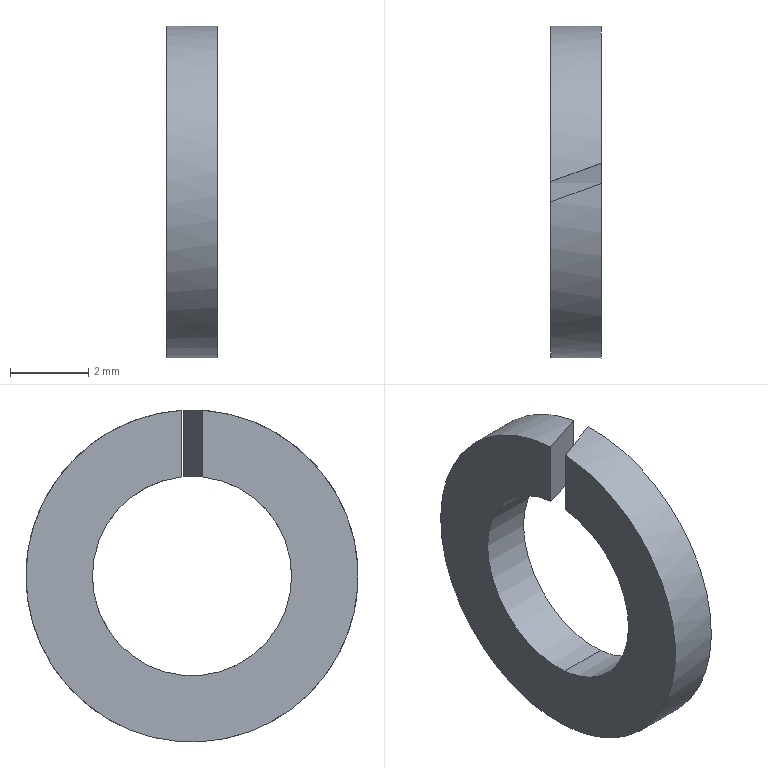Part | STEP file | KS B 1324 - No. 2 - 5 | 1 solid | 8 faces | box 1.3 x 8.5 x 8.5 mm | volume 46.057 mm3 | cylinder 4 | plane 4 | commonest cylinder face diameters 5.1 x2 8.5 x2
STEP:
#1=CARTESIAN_POINT('',(0.,0.,0.));
#2=DIRECTION('',(0.,0.,1.));
#3=DIRECTION('',(1.,0.,0.));
#4=AXIS2_PLACEMENT_3D('',#1,#2,#3);
#5=CARTESIAN_POINT('',(1.3,0.7332,2.442));
#6=VERTEX_POINT('',#5);
#7=CARTESIAN_POINT('',(0.,0.26,2.537));
#8=VERTEX_POINT('',#7);
#9=CARTESIAN_POINT('',(1.3,0.7332,2.442));
#10=CARTESIAN_POINT('',(0.8755,0.5787,2.489));
#11=CARTESIAN_POINT('',(0.4409,0.4205,2.52));
#12=CARTESIAN_POINT('',(0.,0.26,2.537));
#13=(BOUNDED_CURVE()B_SPLINE_CURVE(3,(#9,#10,#11,#12),.UNSPECIFIED.,.F.,.F.)B_SPLINE_CURVE_WITH_KNOTS((4,4),(4.421,4.61),.PIECEWISE_BEZIER_KNOTS.)CURVE()GEOMETRIC_REPRESENTATION_ITEM()RATIONAL_B_SPLINE_CURVE((1.,0.997,0.997,1.))REPRESENTATION_ITEM(''));
#14=CARTESIAN_POINT('',(0.,0.,0.));
#15=DIRECTION('',(1.,0.,0.));
#16=DIRECTION('',(0.,-0.09278,-0.9957));
#17=AXIS2_PLACEMENT_3D('',#14,#15,#16);
#18=CYLINDRICAL_SURFACE('',#17,2.55);
#19=CARTESIAN_POINT('',(2.943,1.3));
#20=CARTESIAN_POINT('',(2.946,1.281));
#21=CARTESIAN_POINT('',(2.951,1.242));
#22=CARTESIAN_POINT('',(2.96,1.184));
#23=CARTESIAN_POINT('',(2.969,1.126));
#24=CARTESIAN_POINT('',(2.977,1.068));
#25=CARTESIAN_POINT('',(2.986,1.009));
#26=CARTESIAN_POINT('',(2.995,0.9509));
#27=CARTESIAN_POINT('',(3.003,0.8922));
#28=CARTESIAN_POINT('',(3.012,0.8334));
#29=CARTESIAN_POINT('',(3.02,0.7744));
#30=CARTESIAN_POINT('',(3.029,0.7153));
#31=CARTESIAN_POINT('',(3.038,0.6562));
#32=CARTESIAN_POINT('',(3.046,0.5969));
#33=CARTESIAN_POINT('',(3.055,0.5375));
#34=CARTESIAN_POINT('',(3.063,0.4781));
#35=CARTESIAN_POINT('',(3.072,0.4185));
#36=CARTESIAN_POINT('',(3.081,0.3589));
#37=CARTESIAN_POINT('',(3.089,0.2992));
#38=CARTESIAN_POINT('',(3.098,0.2395));
#39=CARTESIAN_POINT('',(3.107,0.1797));
#40=CARTESIAN_POINT('',(3.115,0.1198));
#41=CARTESIAN_POINT('',(3.124,0.05993));
#42=CARTESIAN_POINT('',(3.13,0.01998));
#43=CARTESIAN_POINT('',(3.132,0.));
#44=B_SPLINE_CURVE_WITH_KNOTS('',3,(#19,#20,#21,#22,#23,#24,#25,#26,#27,#28,#29,#30,#31,#32,#33,#34,#35,#36,#37,#38,#39,#40,#41,#42,#43),.UNSPECIFIED.,.F.,.F.,(4,1,1,1,1,1,1,1,1,1,1,1,1,1,1,1,1,1,1,1,1,1,4),(4.421,4.429,4.438,4.447,4.455,4.464,4.472,4.481,4.49,4.498,4.507,4.516,4.524,4.533,4.541,4.55,4.559,4.567,4.576,4.584,4.593,4.602,4.61),.QUASI_UNIFORM_KNOTS.);
#45=(GEOMETRIC_REPRESENTATION_CONTEXT(2)PARAMETRIC_REPRESENTATION_CONTEXT()REPRESENTATION_CONTEXT('',''));
#46=DEFINITIONAL_REPRESENTATION('',(#44),#45);
#47=PCURVE('',#18,#46);
#48=CARTESIAN_POINT('',(0.,0.26,0.));
#49=DIRECTION('',(-0.342,0.9397,0.));
#50=DIRECTION('',(0.,0.,1.));
#51=AXIS2_PLACEMENT_3D('',#48,#49,#50);
#52=PLANE('',#51);
#53=CARTESIAN_POINT('',(2.442,1.383));
#54=CARTESIAN_POINT('',(2.489,0.9317));
#55=CARTESIAN_POINT('',(2.52,0.4692));
#56=CARTESIAN_POINT('',(2.537,0.));
#57=(BOUNDED_CURVE()B_SPLINE_CURVE(3,(#53,#54,#55,#56),.UNSPECIFIED.,.F.,.F.)B_SPLINE_CURVE_WITH_KNOTS((4,4),(4.421,4.61),.PIECEWISE_BEZIER_KNOTS.)CURVE()GEOMETRIC_REPRESENTATION_ITEM()RATIONAL_B_SPLINE_CURVE((1.,0.997,0.997,1.))REPRESENTATION_ITEM(''));
#58=(GEOMETRIC_REPRESENTATION_CONTEXT(2)PARAMETRIC_REPRESENTATION_CONTEXT()REPRESENTATION_CONTEXT('',''));
#59=DEFINITIONAL_REPRESENTATION('',(#57),#58);
#60=PCURVE('',#52,#59);
#61=SURFACE_CURVE('',#13,(#47,#60),.PCURVE_S1.);
#62=EDGE_CURVE('',#6,#8,#61,.T.);
#63=ORIENTED_EDGE('',*,*,#62,.F.);
#64=CARTESIAN_POINT('',(1.3,-0.2366,-2.539));
#65=VERTEX_POINT('',#64);
#66=CARTESIAN_POINT('',(1.3,0.,0.));
#67=DIRECTION('',(-1.,0.,0.));
#68=DIRECTION('',(0.,-1.,0.));
#69=AXIS2_PLACEMENT_3D('',#66,#67,#68);
#70=CIRCLE('',#69,2.55);
#71=CARTESIAN_POINT('',(4.805,1.3));
#72=DIRECTION('',(-1.,0.));
#73=VECTOR('',#72,1.);
#74=LINE('',#71,#73);
#75=(GEOMETRIC_REPRESENTATION_CONTEXT(2)PARAMETRIC_REPRESENTATION_CONTEXT()REPRESENTATION_CONTEXT('',''));
#76=DEFINITIONAL_REPRESENTATION('',(#74),#75);
#77=PCURVE('',#18,#76);
#78=CARTESIAN_POINT('',(1.3,0.,0.));
#79=DIRECTION('',(-1.,0.,0.));
#80=DIRECTION('',(0.,0.,1.));
#81=AXIS2_PLACEMENT_3D('',#78,#79,#80);
#82=PLANE('',#81);
#83=CARTESIAN_POINT('',(0.,0.));
#84=DIRECTION('',(0.,-1.));
#85=AXIS2_PLACEMENT_2D('',#83,#84);
#86=CIRCLE('',#85,2.55);
#87=(GEOMETRIC_REPRESENTATION_CONTEXT(2)PARAMETRIC_REPRESENTATION_CONTEXT()REPRESENTATION_CONTEXT('',''));
#88=DEFINITIONAL_REPRESENTATION('',(#86),#87);
#89=PCURVE('',#82,#88);
#90=SURFACE_CURVE('',#70,(#77,#89),.PCURVE_S1.);
#91=EDGE_CURVE('',#6,#65,#90,.T.);
#92=ORIENTED_EDGE('',*,*,#91,.T.);
#93=CARTESIAN_POINT('',(0.,-0.2366,-2.539));
#94=VERTEX_POINT('',#93);
#95=CARTESIAN_POINT('',(0.,-0.2366,-2.539));
#96=DIRECTION('',(1.,0.,0.));
#97=VECTOR('',#96,1.);
#98=LINE('',#95,#97);
#99=CARTESIAN_POINT('',(0.,0.));
#100=DIRECTION('',(0.,1.));
#101=VECTOR('',#100,1.);
#102=LINE('',#99,#101);
#103=(GEOMETRIC_REPRESENTATION_CONTEXT(2)PARAMETRIC_REPRESENTATION_CONTEXT()REPRESENTATION_CONTEXT('',''));
#104=DEFINITIONAL_REPRESENTATION('',(#102),#103);
#105=PCURVE('',#18,#104);
#106=CARTESIAN_POINT('',(0.,0.,0.));
#107=DIRECTION('',(1.,0.,0.));
#108=DIRECTION('',(0.,-0.09278,-0.9957));
#109=AXIS2_PLACEMENT_3D('',#106,#107,#108);
#110=CYLINDRICAL_SURFACE('',#109,2.55);
#111=CARTESIAN_POINT('',(6.283,0.));
#112=DIRECTION('',(0.,1.));
#113=VECTOR('',#112,1.);
#114=LINE('',#111,#113);
#115=(GEOMETRIC_REPRESENTATION_CONTEXT(2)PARAMETRIC_REPRESENTATION_CONTEXT()REPRESENTATION_CONTEXT('',''));
#116=DEFINITIONAL_REPRESENTATION('',(#114),#115);
#117=PCURVE('',#110,#116);
#118=SURFACE_CURVE('',#98,(#105,#117),.PCURVE_S1.);
#119=EDGE_CURVE('',#94,#65,#118,.T.);
#120=ORIENTED_EDGE('',*,*,#119,.F.);
#121=CARTESIAN_POINT('',(0.,0.,0.));
#122=DIRECTION('',(1.,0.,0.));
#123=DIRECTION('',(0.,-1.,0.));
#124=AXIS2_PLACEMENT_3D('',#121,#122,#123);
#125=CIRCLE('',#124,2.55);
#126=CARTESIAN_POINT('',(-1.478,0.));
#127=DIRECTION('',(1.,0.));
#128=VECTOR('',#127,1.);
#129=LINE('',#126,#128);
#130=(GEOMETRIC_REPRESENTATION_CONTEXT(2)PARAMETRIC_REPRESENTATION_CONTEXT()REPRESENTATION_CONTEXT('',''));
#131=DEFINITIONAL_REPRESENTATION('',(#129),#130);
#132=PCURVE('',#18,#131);
#133=CARTESIAN_POINT('',(0.,0.,0.));
#134=DIRECTION('',(-1.,0.,0.));
#135=DIRECTION('',(0.,0.,1.));
#136=AXIS2_PLACEMENT_3D('',#133,#134,#135);
#137=PLANE('',#136);
#138=CARTESIAN_POINT('',(0.,-2.55));
#139=CARTESIAN_POINT('',(-4.417,-2.55));
#140=CARTESIAN_POINT('',(-2.208,1.275));
#141=CARTESIAN_POINT('',(0.,5.1));
#142=CARTESIAN_POINT('',(2.208,1.275));
#143=CARTESIAN_POINT('',(4.417,-2.55));
#144=CARTESIAN_POINT('',(0.,-2.55));
#145=(BOUNDED_CURVE()B_SPLINE_CURVE(2,(#138,#139,#140,#141,#142,#143,#144),.UNSPECIFIED.,.T.,.F.)B_SPLINE_CURVE_WITH_KNOTS((1,2,2,2,2,1),(-2.094,0.,2.094,4.189,6.283,8.378),.UNSPECIFIED.)CURVE()GEOMETRIC_REPRESENTATION_ITEM()RATIONAL_B_SPLINE_CURVE((1.,0.5,1.,0.5,1.,0.5,1.))REPRESENTATION_ITEM(''));
#146=(GEOMETRIC_REPRESENTATION_CONTEXT(2)PARAMETRIC_REPRESENTATION_CONTEXT()REPRESENTATION_CONTEXT('',''));
#147=DEFINITIONAL_REPRESENTATION('',(#145),#146);
#148=PCURVE('',#137,#147);
#149=SURFACE_CURVE('',#125,(#132,#148),.PCURVE_S1.);
#150=EDGE_CURVE('',#94,#8,#149,.T.);
#151=ORIENTED_EDGE('',*,*,#150,.T.);
#152=EDGE_LOOP('',(#63,#92,#120,#151));
#153=FACE_BOUND('',#152,.F.);
#154=ADVANCED_FACE('',(#153),#18,.F.);
#155=CARTESIAN_POINT('',(0.,-0.2366,-4.243));
#156=VERTEX_POINT('',#155);
#157=CARTESIAN_POINT('',(0.,-0.26,4.242));
#158=VERTEX_POINT('',#157);
#159=CARTESIAN_POINT('',(0.,0.,0.));
#160=DIRECTION('',(-1.,0.,0.));
#161=DIRECTION('',(0.,-1.,0.));
#162=AXIS2_PLACEMENT_3D('',#159,#160,#161);
#163=CIRCLE('',#162,4.25);
#164=CARTESIAN_POINT('',(0.,0.,0.));
#165=DIRECTION('',(1.,0.,0.));
#166=DIRECTION('',(0.,-0.05567,-0.9984));
#167=AXIS2_PLACEMENT_3D('',#164,#165,#166);
#168=CYLINDRICAL_SURFACE('',#167,4.25);
#169=CARTESIAN_POINT('',(11.051,0.));
#170=DIRECTION('',(-1.,0.));
#171=VECTOR('',#170,1.);
#172=LINE('',#169,#171);
#173=(GEOMETRIC_REPRESENTATION_CONTEXT(2)PARAMETRIC_REPRESENTATION_CONTEXT()REPRESENTATION_CONTEXT('',''));
#174=DEFINITIONAL_REPRESENTATION('',(#172),#173);
#175=PCURVE('',#168,#174);
#176=CARTESIAN_POINT('',(0.,0.));
#177=DIRECTION('',(0.,-1.));
#178=AXIS2_PLACEMENT_2D('',#176,#177);
#179=CIRCLE('',#178,4.25);
#180=(GEOMETRIC_REPRESENTATION_CONTEXT(2)PARAMETRIC_REPRESENTATION_CONTEXT()REPRESENTATION_CONTEXT('',''));
#181=DEFINITIONAL_REPRESENTATION('',(#179),#180);
#182=PCURVE('',#137,#181);
#183=SURFACE_CURVE('',#163,(#175,#182),.PCURVE_S1.);
#184=EDGE_CURVE('',#156,#158,#183,.T.);
#185=ORIENTED_EDGE('',*,*,#184,.F.);
#186=CARTESIAN_POINT('',(1.3,-0.2366,-4.243));
#187=VERTEX_POINT('',#186);
#188=CARTESIAN_POINT('',(0.,-0.2366,-4.243));
#189=DIRECTION('',(1.,0.,0.));
#190=VECTOR('',#189,1.);
#191=LINE('',#188,#190);
#192=CARTESIAN_POINT('',(6.283,0.));
#193=DIRECTION('',(0.,1.));
#194=VECTOR('',#193,1.);
#195=LINE('',#192,#194);
#196=(GEOMETRIC_REPRESENTATION_CONTEXT(2)PARAMETRIC_REPRESENTATION_CONTEXT()REPRESENTATION_CONTEXT('',''));
#197=DEFINITIONAL_REPRESENTATION('',(#195),#196);
#198=PCURVE('',#168,#197);
#199=CARTESIAN_POINT('',(0.,0.,0.));
#200=DIRECTION('',(1.,0.,0.));
#201=DIRECTION('',(0.,-0.05567,-0.9984));
#202=AXIS2_PLACEMENT_3D('',#199,#200,#201);
#203=CYLINDRICAL_SURFACE('',#202,4.25);
#204=CARTESIAN_POINT('',(0.,0.));
#205=DIRECTION('',(0.,1.));
#206=VECTOR('',#205,1.);
#207=LINE('',#204,#206);
#208=(GEOMETRIC_REPRESENTATION_CONTEXT(2)PARAMETRIC_REPRESENTATION_CONTEXT()REPRESENTATION_CONTEXT('',''));
#209=DEFINITIONAL_REPRESENTATION('',(#207),#208);
#210=PCURVE('',#203,#209);
#211=SURFACE_CURVE('',#191,(#198,#210),.PCURVE_S1.);
#212=EDGE_CURVE('',#156,#187,#211,.T.);
#213=ORIENTED_EDGE('',*,*,#212,.T.);
#214=CARTESIAN_POINT('',(1.3,0.2132,4.245));
#215=VERTEX_POINT('',#214);
#216=CARTESIAN_POINT('',(1.3,0.,0.));
#217=DIRECTION('',(-1.,0.,0.));
#218=DIRECTION('',(0.,-1.,0.));
#219=AXIS2_PLACEMENT_3D('',#216,#217,#218);
#220=CIRCLE('',#219,4.25);
#221=CARTESIAN_POINT('',(11.051,1.3));
#222=DIRECTION('',(-1.,0.));
#223=VECTOR('',#222,1.);
#224=LINE('',#221,#223);
#225=(GEOMETRIC_REPRESENTATION_CONTEXT(2)PARAMETRIC_REPRESENTATION_CONTEXT()REPRESENTATION_CONTEXT('',''));
#226=DEFINITIONAL_REPRESENTATION('',(#224),#225);
#227=PCURVE('',#168,#226);
#228=CARTESIAN_POINT('',(0.,0.));
#229=DIRECTION('',(0.,-1.));
#230=AXIS2_PLACEMENT_2D('',#228,#229);
#231=CIRCLE('',#230,4.25);
#232=(GEOMETRIC_REPRESENTATION_CONTEXT(2)PARAMETRIC_REPRESENTATION_CONTEXT()REPRESENTATION_CONTEXT('',''));
#233=DEFINITIONAL_REPRESENTATION('',(#231),#232);
#234=PCURVE('',#82,#233);
#235=SURFACE_CURVE('',#220,(#227,#234),.PCURVE_S1.);
#236=EDGE_CURVE('',#187,#215,#235,.T.);
#237=ORIENTED_EDGE('',*,*,#236,.T.);
#238=CARTESIAN_POINT('',(1.3,0.2132,4.245));
#239=CARTESIAN_POINT('',(0.8668,0.05547,4.253));
#240=CARTESIAN_POINT('',(0.433,-0.1024,4.252));
#241=CARTESIAN_POINT('',(0.,-0.26,4.242));
#242=(BOUNDED_CURVE()B_SPLINE_CURVE(3,(#238,#239,#240,#241),.UNSPECIFIED.,.F.,.F.)B_SPLINE_CURVE_WITH_KNOTS((4,4),(4.662,4.774),.PIECEWISE_BEZIER_KNOTS.)CURVE()GEOMETRIC_REPRESENTATION_ITEM()RATIONAL_B_SPLINE_CURVE((1.,0.999,0.999,1.))REPRESENTATION_ITEM(''));
#243=CARTESIAN_POINT('',(3.147,1.3));
#244=CARTESIAN_POINT('',(3.149,1.28));
#245=CARTESIAN_POINT('',(3.152,1.241));
#246=CARTESIAN_POINT('',(3.157,1.182));
#247=CARTESIAN_POINT('',(3.162,1.123));
#248=CARTESIAN_POINT('',(3.167,1.064));
#249=CARTESIAN_POINT('',(3.172,1.005));
#250=CARTESIAN_POINT('',(3.177,0.9456));
#251=CARTESIAN_POINT('',(3.183,0.8864));
#252=CARTESIAN_POINT('',(3.188,0.8273));
#253=CARTESIAN_POINT('',(3.193,0.7682));
#254=CARTESIAN_POINT('',(3.198,0.709));
#255=CARTESIAN_POINT('',(3.203,0.6499));
#256=CARTESIAN_POINT('',(3.208,0.5908));
#257=CARTESIAN_POINT('',(3.213,0.5316));
#258=CARTESIAN_POINT('',(3.218,0.4725));
#259=CARTESIAN_POINT('',(3.223,0.4134));
#260=CARTESIAN_POINT('',(3.228,0.3543));
#261=CARTESIAN_POINT('',(3.233,0.2952));
#262=CARTESIAN_POINT('',(3.238,0.2361));
#263=CARTESIAN_POINT('',(3.243,0.177));
#264=CARTESIAN_POINT('',(3.248,0.118));
#265=CARTESIAN_POINT('',(3.253,0.05899));
#266=CARTESIAN_POINT('',(3.257,0.01966));
#267=CARTESIAN_POINT('',(3.259,0.));
#268=B_SPLINE_CURVE_WITH_KNOTS('',3,(#243,#244,#245,#246,#247,#248,#249,#250,#251,#252,#253,#254,#255,#256,#257,#258,#259,#260,#261,#262,#263,#264,#265,#266,#267),.UNSPECIFIED.,.F.,.F.,(4,1,1,1,1,1,1,1,1,1,1,1,1,1,1,1,1,1,1,1,1,1,4),(4.662,4.667,4.672,4.677,4.682,4.688,4.693,4.698,4.703,4.708,4.713,4.718,4.723,4.728,4.733,4.738,4.743,4.748,4.753,4.758,4.763,4.769,4.774),.QUASI_UNIFORM_KNOTS.);
#269=(GEOMETRIC_REPRESENTATION_CONTEXT(2)PARAMETRIC_REPRESENTATION_CONTEXT()REPRESENTATION_CONTEXT('',''));
#270=DEFINITIONAL_REPRESENTATION('',(#268),#269);
#271=PCURVE('',#168,#270);
#272=CARTESIAN_POINT('',(1.3,0.2132,0.));
#273=DIRECTION('',(0.342,-0.9397,0.));
#274=DIRECTION('',(0.,0.,-1.));
#275=AXIS2_PLACEMENT_3D('',#272,#273,#274);
#276=PLANE('',#275);
#277=CARTESIAN_POINT('',(-4.245,0.));
#278=CARTESIAN_POINT('',(-4.253,-0.461));
#279=CARTESIAN_POINT('',(-4.252,-0.9227));
#280=CARTESIAN_POINT('',(-4.242,-1.383));
#281=(BOUNDED_CURVE()B_SPLINE_CURVE(3,(#277,#278,#279,#280),.UNSPECIFIED.,.F.,.F.)B_SPLINE_CURVE_WITH_KNOTS((4,4),(4.662,4.774),.PIECEWISE_BEZIER_KNOTS.)CURVE()GEOMETRIC_REPRESENTATION_ITEM()RATIONAL_B_SPLINE_CURVE((1.,0.999,0.999,1.))REPRESENTATION_ITEM(''));
#282=(GEOMETRIC_REPRESENTATION_CONTEXT(2)PARAMETRIC_REPRESENTATION_CONTEXT()REPRESENTATION_CONTEXT('',''));
#283=DEFINITIONAL_REPRESENTATION('',(#281),#282);
#284=PCURVE('',#276,#283);
#285=SURFACE_CURVE('',#242,(#271,#284),.PCURVE_S1.);
#286=EDGE_CURVE('',#215,#158,#285,.T.);
#287=ORIENTED_EDGE('',*,*,#286,.T.);
#288=EDGE_LOOP('',(#185,#213,#237,#287));
#289=FACE_BOUND('',#288,.T.);
#290=ADVANCED_FACE('',(#289),#168,.T.);
#291=CARTESIAN_POINT('',(0.,-0.26,2.537));
#292=VERTEX_POINT('',#291);
#293=CARTESIAN_POINT('',(0.,-0.26,0.));
#294=DIRECTION('',(0.,0.,-1.));
#295=VECTOR('',#294,1.);
#296=LINE('',#293,#295);
#297=CARTESIAN_POINT('',(0.,-0.26));
#298=DIRECTION('',(-1.,0.));
#299=VECTOR('',#298,1.);
#300=LINE('',#297,#299);
#301=(GEOMETRIC_REPRESENTATION_CONTEXT(2)PARAMETRIC_REPRESENTATION_CONTEXT()REPRESENTATION_CONTEXT('',''));
#302=DEFINITIONAL_REPRESENTATION('',(#300),#301);
#303=PCURVE('',#137,#302);
#304=CARTESIAN_POINT('',(0.,-1.383));
#305=DIRECTION('',(1.,0.));
#306=VECTOR('',#305,1.);
#307=LINE('',#304,#306);
#308=(GEOMETRIC_REPRESENTATION_CONTEXT(2)PARAMETRIC_REPRESENTATION_CONTEXT()REPRESENTATION_CONTEXT('',''));
#309=DEFINITIONAL_REPRESENTATION('',(#307),#308);
#310=PCURVE('',#276,#309);
#311=SURFACE_CURVE('',#296,(#303,#310),.PCURVE_S1.);
#312=EDGE_CURVE('',#158,#292,#311,.T.);
#313=ORIENTED_EDGE('',*,*,#312,.T.);
#314=CARTESIAN_POINT('',(0.,0.,0.));
#315=DIRECTION('',(1.,0.,0.));
#316=DIRECTION('',(0.,-1.,0.));
#317=AXIS2_PLACEMENT_3D('',#314,#315,#316);
#318=CIRCLE('',#317,2.55);
#319=CARTESIAN_POINT('',(0.,-2.55));
#320=CARTESIAN_POINT('',(-4.417,-2.55));
#321=CARTESIAN_POINT('',(-2.208,1.275));
#322=CARTESIAN_POINT('',(0.,5.1));
#323=CARTESIAN_POINT('',(2.208,1.275));
#324=CARTESIAN_POINT('',(4.417,-2.55));
#325=CARTESIAN_POINT('',(0.,-2.55));
#326=(BOUNDED_CURVE()B_SPLINE_CURVE(2,(#319,#320,#321,#322,#323,#324,#325),.UNSPECIFIED.,.T.,.F.)B_SPLINE_CURVE_WITH_KNOTS((1,2,2,2,2,1),(-2.094,0.,2.094,4.189,6.283,8.378),.UNSPECIFIED.)CURVE()GEOMETRIC_REPRESENTATION_ITEM()RATIONAL_B_SPLINE_CURVE((1.,0.5,1.,0.5,1.,0.5,1.))REPRESENTATION_ITEM(''));
#327=(GEOMETRIC_REPRESENTATION_CONTEXT(2)PARAMETRIC_REPRESENTATION_CONTEXT()REPRESENTATION_CONTEXT('',''));
#328=DEFINITIONAL_REPRESENTATION('',(#326),#327);
#329=PCURVE('',#137,#328);
#330=CARTESIAN_POINT('',(-1.478,0.));
#331=DIRECTION('',(1.,0.));
#332=VECTOR('',#331,1.);
#333=LINE('',#330,#332);
#334=(GEOMETRIC_REPRESENTATION_CONTEXT(2)PARAMETRIC_REPRESENTATION_CONTEXT()REPRESENTATION_CONTEXT('',''));
#335=DEFINITIONAL_REPRESENTATION('',(#333),#334);
#336=PCURVE('',#110,#335);
#337=SURFACE_CURVE('',#318,(#329,#336),.PCURVE_S1.);
#338=EDGE_CURVE('',#292,#94,#337,.T.);
#339=ORIENTED_EDGE('',*,*,#338,.T.);
#340=ORIENTED_EDGE('',*,*,#150,.T.);
#341=CARTESIAN_POINT('',(0.,0.26,4.242));
#342=VERTEX_POINT('',#341);
#343=CARTESIAN_POINT('',(0.,0.26,0.));
#344=DIRECTION('',(0.,0.,1.));
#345=VECTOR('',#344,1.);
#346=LINE('',#343,#345);
#347=CARTESIAN_POINT('',(0.,0.26));
#348=DIRECTION('',(1.,0.));
#349=VECTOR('',#348,1.);
#350=LINE('',#347,#349);
#351=(GEOMETRIC_REPRESENTATION_CONTEXT(2)PARAMETRIC_REPRESENTATION_CONTEXT()REPRESENTATION_CONTEXT('',''));
#352=DEFINITIONAL_REPRESENTATION('',(#350),#351);
#353=PCURVE('',#137,#352);
#354=CARTESIAN_POINT('',(0.,0.));
#355=DIRECTION('',(1.,0.));
#356=VECTOR('',#355,1.);
#357=LINE('',#354,#356);
#358=(GEOMETRIC_REPRESENTATION_CONTEXT(2)PARAMETRIC_REPRESENTATION_CONTEXT()REPRESENTATION_CONTEXT('',''));
#359=DEFINITIONAL_REPRESENTATION('',(#357),#358);
#360=PCURVE('',#52,#359);
#361=SURFACE_CURVE('',#346,(#353,#360),.PCURVE_S1.);
#362=EDGE_CURVE('',#8,#342,#361,.T.);
#363=ORIENTED_EDGE('',*,*,#362,.T.);
#364=CARTESIAN_POINT('',(0.,0.,0.));
#365=DIRECTION('',(-1.,0.,0.));
#366=DIRECTION('',(0.,-1.,0.));
#367=AXIS2_PLACEMENT_3D('',#364,#365,#366);
#368=CIRCLE('',#367,4.25);
#369=CARTESIAN_POINT('',(0.,0.));
#370=DIRECTION('',(0.,-1.));
#371=AXIS2_PLACEMENT_2D('',#369,#370);
#372=CIRCLE('',#371,4.25);
#373=(GEOMETRIC_REPRESENTATION_CONTEXT(2)PARAMETRIC_REPRESENTATION_CONTEXT()REPRESENTATION_CONTEXT('',''));
#374=DEFINITIONAL_REPRESENTATION('',(#372),#373);
#375=PCURVE('',#137,#374);
#376=CARTESIAN_POINT('',(4.768,0.));
#377=DIRECTION('',(-1.,0.));
#378=VECTOR('',#377,1.);
#379=LINE('',#376,#378);
#380=(GEOMETRIC_REPRESENTATION_CONTEXT(2)PARAMETRIC_REPRESENTATION_CONTEXT()REPRESENTATION_CONTEXT('',''));
#381=DEFINITIONAL_REPRESENTATION('',(#379),#380);
#382=PCURVE('',#203,#381);
#383=SURFACE_CURVE('',#368,(#375,#382),.PCURVE_S1.);
#384=EDGE_CURVE('',#342,#156,#383,.T.);
#385=ORIENTED_EDGE('',*,*,#384,.T.);
#386=ORIENTED_EDGE('',*,*,#184,.T.);
#387=EDGE_LOOP('',(#313,#339,#340,#363,#385,#386));
#388=FACE_BOUND('',#387,.T.);
#389=ADVANCED_FACE('',(#388),#137,.T.);
#390=ORIENTED_EDGE('',*,*,#212,.F.);
#391=ORIENTED_EDGE('',*,*,#384,.F.);
#392=CARTESIAN_POINT('',(1.3,0.7332,4.186));
#393=VERTEX_POINT('',#392);
#394=CARTESIAN_POINT('',(0.,0.26,4.242));
#395=CARTESIAN_POINT('',(0.436,0.4187,4.232));
#396=CARTESIAN_POINT('',(0.8698,0.5766,4.214));
#397=CARTESIAN_POINT('',(1.3,0.7332,4.186));
#398=(BOUNDED_CURVE()B_SPLINE_CURVE(3,(#394,#395,#396,#397),.UNSPECIFIED.,.F.,.F.)B_SPLINE_CURVE_WITH_KNOTS((4,4),(1.632,1.744),.PIECEWISE_BEZIER_KNOTS.)CURVE()GEOMETRIC_REPRESENTATION_ITEM()RATIONAL_B_SPLINE_CURVE((1.,0.999,0.999,1.))REPRESENTATION_ITEM(''));
#399=CARTESIAN_POINT('',(3.136,0.));
#400=CARTESIAN_POINT('',(3.134,0.0198));
#401=CARTESIAN_POINT('',(3.131,0.05938));
#402=CARTESIAN_POINT('',(3.126,0.1188));
#403=CARTESIAN_POINT('',(3.121,0.1781));
#404=CARTESIAN_POINT('',(3.116,0.2375));
#405=CARTESIAN_POINT('',(3.111,0.2968));
#406=CARTESIAN_POINT('',(3.105,0.3561));
#407=CARTESIAN_POINT('',(3.1,0.4153));
#408=CARTESIAN_POINT('',(3.095,0.4746));
#409=CARTESIAN_POINT('',(3.09,0.5338));
#410=CARTESIAN_POINT('',(3.085,0.593));
#411=CARTESIAN_POINT('',(3.08,0.6522));
#412=CARTESIAN_POINT('',(3.075,0.7113));
#413=CARTESIAN_POINT('',(3.07,0.7704));
#414=CARTESIAN_POINT('',(3.065,0.8294));
#415=CARTESIAN_POINT('',(3.06,0.8884));
#416=CARTESIAN_POINT('',(3.054,0.9474));
#417=CARTESIAN_POINT('',(3.049,1.006));
#418=CARTESIAN_POINT('',(3.044,1.065));
#419=CARTESIAN_POINT('',(3.039,1.124));
#420=CARTESIAN_POINT('',(3.034,1.183));
#421=CARTESIAN_POINT('',(3.029,1.241));
#422=CARTESIAN_POINT('',(3.026,1.28));
#423=CARTESIAN_POINT('',(3.024,1.3));
#424=B_SPLINE_CURVE_WITH_KNOTS('',3,(#399,#400,#401,#402,#403,#404,#405,#406,#407,#408,#409,#410,#411,#412,#413,#414,#415,#416,#417,#418,#419,#420,#421,#422,#423),.UNSPECIFIED.,.F.,.F.,(4,1,1,1,1,1,1,1,1,1,1,1,1,1,1,1,1,1,1,1,1,1,4),(1.632,1.637,1.642,1.647,1.652,1.658,1.663,1.668,1.673,1.678,1.683,1.688,1.693,1.698,1.703,1.708,1.714,1.719,1.724,1.729,1.734,1.739,1.744),.QUASI_UNIFORM_KNOTS.);
#425=(GEOMETRIC_REPRESENTATION_CONTEXT(2)PARAMETRIC_REPRESENTATION_CONTEXT()REPRESENTATION_CONTEXT('',''));
#426=DEFINITIONAL_REPRESENTATION('',(#424),#425);
#427=PCURVE('',#203,#426);
#428=CARTESIAN_POINT('',(4.242,0.));
#429=CARTESIAN_POINT('',(4.232,0.464));
#430=CARTESIAN_POINT('',(4.214,0.9256));
#431=CARTESIAN_POINT('',(4.186,1.383));
#432=(BOUNDED_CURVE()B_SPLINE_CURVE(3,(#428,#429,#430,#431),.UNSPECIFIED.,.F.,.F.)B_SPLINE_CURVE_WITH_KNOTS((4,4),(1.632,1.744),.PIECEWISE_BEZIER_KNOTS.)CURVE()GEOMETRIC_REPRESENTATION_ITEM()RATIONAL_B_SPLINE_CURVE((1.,0.999,0.999,1.))REPRESENTATION_ITEM(''));
#433=(GEOMETRIC_REPRESENTATION_CONTEXT(2)PARAMETRIC_REPRESENTATION_CONTEXT()REPRESENTATION_CONTEXT('',''));
#434=DEFINITIONAL_REPRESENTATION('',(#432),#433);
#435=PCURVE('',#52,#434);
#436=SURFACE_CURVE('',#398,(#427,#435),.PCURVE_S1.);
#437=EDGE_CURVE('',#342,#393,#436,.T.);
#438=ORIENTED_EDGE('',*,*,#437,.T.);
#439=CARTESIAN_POINT('',(1.3,0.,0.));
#440=DIRECTION('',(-1.,0.,0.));
#441=DIRECTION('',(0.,-1.,0.));
#442=AXIS2_PLACEMENT_3D('',#439,#440,#441);
#443=CIRCLE('',#442,4.25);
#444=CARTESIAN_POINT('',(4.768,1.3));
#445=DIRECTION('',(-1.,0.));
#446=VECTOR('',#445,1.);
#447=LINE('',#444,#446);
#448=(GEOMETRIC_REPRESENTATION_CONTEXT(2)PARAMETRIC_REPRESENTATION_CONTEXT()REPRESENTATION_CONTEXT('',''));
#449=DEFINITIONAL_REPRESENTATION('',(#447),#448);
#450=PCURVE('',#203,#449);
#451=CARTESIAN_POINT('',(0.,0.));
#452=DIRECTION('',(0.,-1.));
#453=AXIS2_PLACEMENT_2D('',#451,#452);
#454=CIRCLE('',#453,4.25);
#455=(GEOMETRIC_REPRESENTATION_CONTEXT(2)PARAMETRIC_REPRESENTATION_CONTEXT()REPRESENTATION_CONTEXT('',''));
#456=DEFINITIONAL_REPRESENTATION('',(#454),#455);
#457=PCURVE('',#82,#456);
#458=SURFACE_CURVE('',#443,(#450,#457),.PCURVE_S1.);
#459=EDGE_CURVE('',#393,#187,#458,.T.);
#460=ORIENTED_EDGE('',*,*,#459,.T.);
#461=EDGE_LOOP('',(#390,#391,#438,#460));
#462=FACE_BOUND('',#461,.T.);
#463=ADVANCED_FACE('',(#462),#203,.T.);
#464=CARTESIAN_POINT('',(1.3,0.2132,2.541));
#465=VERTEX_POINT('',#464);
#466=CARTESIAN_POINT('',(1.3,0.,0.));
#467=DIRECTION('',(-1.,0.,0.));
#468=DIRECTION('',(0.,-1.,0.));
#469=AXIS2_PLACEMENT_3D('',#466,#467,#468);
#470=CIRCLE('',#469,2.55);
#471=CARTESIAN_POINT('',(11.088,1.3));
#472=DIRECTION('',(-1.,0.));
#473=VECTOR('',#472,1.);
#474=LINE('',#471,#473);
#475=(GEOMETRIC_REPRESENTATION_CONTEXT(2)PARAMETRIC_REPRESENTATION_CONTEXT()REPRESENTATION_CONTEXT('',''));
#476=DEFINITIONAL_REPRESENTATION('',(#474),#475);
#477=PCURVE('',#110,#476);
#478=CARTESIAN_POINT('',(0.,0.));
#479=DIRECTION('',(0.,-1.));
#480=AXIS2_PLACEMENT_2D('',#478,#479);
#481=CIRCLE('',#480,2.55);
#482=(GEOMETRIC_REPRESENTATION_CONTEXT(2)PARAMETRIC_REPRESENTATION_CONTEXT()REPRESENTATION_CONTEXT('',''));
#483=DEFINITIONAL_REPRESENTATION('',(#481),#482);
#484=PCURVE('',#82,#483);
#485=SURFACE_CURVE('',#470,(#477,#484),.PCURVE_S1.);
#486=EDGE_CURVE('',#65,#465,#485,.T.);
#487=ORIENTED_EDGE('',*,*,#486,.T.);
#488=CARTESIAN_POINT('',(0.,-0.26,2.537));
#489=CARTESIAN_POINT('',(0.4323,-0.1026,2.553));
#490=CARTESIAN_POINT('',(0.8669,0.05553,2.554));
#491=CARTESIAN_POINT('',(1.3,0.2132,2.541));
#492=(BOUNDED_CURVE()B_SPLINE_CURVE(3,(#488,#489,#490,#491),.UNSPECIFIED.,.F.,.F.)B_SPLINE_CURVE_WITH_KNOTS((4,4),(1.469,1.654),.PIECEWISE_BEZIER_KNOTS.)CURVE()GEOMETRIC_REPRESENTATION_ITEM()RATIONAL_B_SPLINE_CURVE((1.,0.9971,0.9971,1.))REPRESENTATION_ITEM(''));
#493=CARTESIAN_POINT('',(3.337,0.));
#494=CARTESIAN_POINT('',(3.334,0.0196));
#495=CARTESIAN_POINT('',(3.328,0.05881));
#496=CARTESIAN_POINT('',(3.32,0.1177));
#497=CARTESIAN_POINT('',(3.311,0.1767));
#498=CARTESIAN_POINT('',(3.303,0.2357));
#499=CARTESIAN_POINT('',(3.294,0.2947));
#500=CARTESIAN_POINT('',(3.286,0.3538));
#501=CARTESIAN_POINT('',(3.278,0.4129));
#502=CARTESIAN_POINT('',(3.269,0.4721));
#503=CARTESIAN_POINT('',(3.261,0.5313));
#504=CARTESIAN_POINT('',(3.252,0.5905));
#505=CARTESIAN_POINT('',(3.244,0.6497));
#506=CARTESIAN_POINT('',(3.235,0.7089));
#507=CARTESIAN_POINT('',(3.227,0.7682));
#508=CARTESIAN_POINT('',(3.218,0.8274));
#509=CARTESIAN_POINT('',(3.21,0.8866));
#510=CARTESIAN_POINT('',(3.201,0.9457));
#511=CARTESIAN_POINT('',(3.193,1.005));
#512=CARTESIAN_POINT('',(3.185,1.064));
#513=CARTESIAN_POINT('',(3.176,1.123));
#514=CARTESIAN_POINT('',(3.168,1.182));
#515=CARTESIAN_POINT('',(3.159,1.241));
#516=CARTESIAN_POINT('',(3.154,1.28));
#517=CARTESIAN_POINT('',(3.151,1.3));
#518=B_SPLINE_CURVE_WITH_KNOTS('',3,(#493,#494,#495,#496,#497,#498,#499,#500,#501,#502,#503,#504,#505,#506,#507,#508,#509,#510,#511,#512,#513,#514,#515,#516,#517),.UNSPECIFIED.,.F.,.F.,(4,1,1,1,1,1,1,1,1,1,1,1,1,1,1,1,1,1,1,1,1,1,4),(1.469,1.477,1.486,1.494,1.502,1.511,1.519,1.528,1.536,1.545,1.553,1.562,1.57,1.578,1.587,1.595,1.604,1.612,1.621,1.629,1.638,1.646,1.654),.QUASI_UNIFORM_KNOTS.);
#519=(GEOMETRIC_REPRESENTATION_CONTEXT(2)PARAMETRIC_REPRESENTATION_CONTEXT()REPRESENTATION_CONTEXT('',''));
#520=DEFINITIONAL_REPRESENTATION('',(#518),#519);
#521=PCURVE('',#110,#520);
#522=CARTESIAN_POINT('',(-2.537,-1.383));
#523=CARTESIAN_POINT('',(-2.553,-0.9233));
#524=CARTESIAN_POINT('',(-2.554,-0.4609));
#525=CARTESIAN_POINT('',(-2.541,0.));
#526=(BOUNDED_CURVE()B_SPLINE_CURVE(3,(#522,#523,#524,#525),.UNSPECIFIED.,.F.,.F.)B_SPLINE_CURVE_WITH_KNOTS((4,4),(1.469,1.654),.PIECEWISE_BEZIER_KNOTS.)CURVE()GEOMETRIC_REPRESENTATION_ITEM()RATIONAL_B_SPLINE_CURVE((1.,0.9971,0.9971,1.))REPRESENTATION_ITEM(''));
#527=(GEOMETRIC_REPRESENTATION_CONTEXT(2)PARAMETRIC_REPRESENTATION_CONTEXT()REPRESENTATION_CONTEXT('',''));
#528=DEFINITIONAL_REPRESENTATION('',(#526),#527);
#529=PCURVE('',#276,#528);
#530=SURFACE_CURVE('',#492,(#521,#529),.PCURVE_S1.);
#531=EDGE_CURVE('',#292,#465,#530,.T.);
#532=ORIENTED_EDGE('',*,*,#531,.F.);
#533=ORIENTED_EDGE('',*,*,#338,.T.);
#534=ORIENTED_EDGE('',*,*,#119,.T.);
#535=EDGE_LOOP('',(#487,#532,#533,#534));
#536=FACE_BOUND('',#535,.F.);
#537=ADVANCED_FACE('',(#536),#110,.F.);
#538=CARTESIAN_POINT('',(1.3,0.2132,0.));
#539=DIRECTION('',(0.,0.,1.));
#540=VECTOR('',#539,1.);
#541=LINE('',#538,#540);
#542=CARTESIAN_POINT('',(0.,0.2132));
#543=DIRECTION('',(1.,0.));
#544=VECTOR('',#543,1.);
#545=LINE('',#542,#544);
#546=(GEOMETRIC_REPRESENTATION_CONTEXT(2)PARAMETRIC_REPRESENTATION_CONTEXT()REPRESENTATION_CONTEXT('',''));
#547=DEFINITIONAL_REPRESENTATION('',(#545),#546);
#548=PCURVE('',#82,#547);
#549=CARTESIAN_POINT('',(0.,0.));
#550=DIRECTION('',(-1.,0.));
#551=VECTOR('',#550,1.);
#552=LINE('',#549,#551);
#553=(GEOMETRIC_REPRESENTATION_CONTEXT(2)PARAMETRIC_REPRESENTATION_CONTEXT()REPRESENTATION_CONTEXT('',''));
#554=DEFINITIONAL_REPRESENTATION('',(#552),#553);
#555=PCURVE('',#276,#554);
#556=SURFACE_CURVE('',#541,(#548,#555),.PCURVE_S1.);
#557=EDGE_CURVE('',#465,#215,#556,.T.);
#558=ORIENTED_EDGE('',*,*,#557,.T.);
#559=ORIENTED_EDGE('',*,*,#236,.F.);
#560=ORIENTED_EDGE('',*,*,#459,.F.);
#561=CARTESIAN_POINT('',(1.3,0.7332,0.));
#562=DIRECTION('',(0.,0.,-1.));
#563=VECTOR('',#562,1.);
#564=LINE('',#561,#563);
#565=CARTESIAN_POINT('',(0.,0.7332));
#566=DIRECTION('',(-1.,0.));
#567=VECTOR('',#566,1.);
#568=LINE('',#565,#567);
#569=(GEOMETRIC_REPRESENTATION_CONTEXT(2)PARAMETRIC_REPRESENTATION_CONTEXT()REPRESENTATION_CONTEXT('',''));
#570=DEFINITIONAL_REPRESENTATION('',(#568),#569);
#571=PCURVE('',#82,#570);
#572=CARTESIAN_POINT('',(0.,1.383));
#573=DIRECTION('',(-1.,0.));
#574=VECTOR('',#573,1.);
#575=LINE('',#572,#574);
#576=(GEOMETRIC_REPRESENTATION_CONTEXT(2)PARAMETRIC_REPRESENTATION_CONTEXT()REPRESENTATION_CONTEXT('',''));
#577=DEFINITIONAL_REPRESENTATION('',(#575),#576);
#578=PCURVE('',#52,#577);
#579=SURFACE_CURVE('',#564,(#571,#578),.PCURVE_S1.);
#580=EDGE_CURVE('',#393,#6,#579,.T.);
#581=ORIENTED_EDGE('',*,*,#580,.T.);
#582=ORIENTED_EDGE('',*,*,#91,.T.);
#583=ORIENTED_EDGE('',*,*,#486,.T.);
#584=EDGE_LOOP('',(#558,#559,#560,#581,#582,#583));
#585=FACE_BOUND('',#584,.T.);
#586=ADVANCED_FACE('',(#585),#82,.F.);
#587=ORIENTED_EDGE('',*,*,#531,.F.);
#588=ORIENTED_EDGE('',*,*,#312,.F.);
#589=ORIENTED_EDGE('',*,*,#286,.F.);
#590=ORIENTED_EDGE('',*,*,#557,.F.);
#591=EDGE_LOOP('',(#587,#588,#589,#590));
#592=FACE_BOUND('',#591,.T.);
#593=ADVANCED_FACE('',(#592),#276,.F.);
#594=ORIENTED_EDGE('',*,*,#62,.F.);
#595=ORIENTED_EDGE('',*,*,#580,.F.);
#596=ORIENTED_EDGE('',*,*,#437,.F.);
#597=ORIENTED_EDGE('',*,*,#362,.F.);
#598=EDGE_LOOP('',(#594,#595,#596,#597));
#599=FACE_BOUND('',#598,.T.);
#600=ADVANCED_FACE('',(#599),#52,.F.);
#601=CLOSED_SHELL('',(#154,#290,#389,#463,#537,#586,#593,#600));
#602=MANIFOLD_SOLID_BREP('',#601);
#603=(LENGTH_UNIT()NAMED_UNIT(*)SI_UNIT(.MILLI.,.METRE.));
#604=UNCERTAINTY_MEASURE_WITH_UNIT(LENGTH_MEASURE(0.0000001),#603,'','');
#605=(NAMED_UNIT(*)PLANE_ANGLE_UNIT()SI_UNIT($,.RADIAN.));
#606=(NAMED_UNIT(*)SI_UNIT($,.STERADIAN.)SOLID_ANGLE_UNIT());
#607=(GEOMETRIC_REPRESENTATION_CONTEXT(3)GLOBAL_UNCERTAINTY_ASSIGNED_CONTEXT((#604))GLOBAL_UNIT_ASSIGNED_CONTEXT((#603,#605,#606))REPRESENTATION_CONTEXT('',''));
#608=ADVANCED_BREP_SHAPE_REPRESENTATION('',(#4,#602),#607);